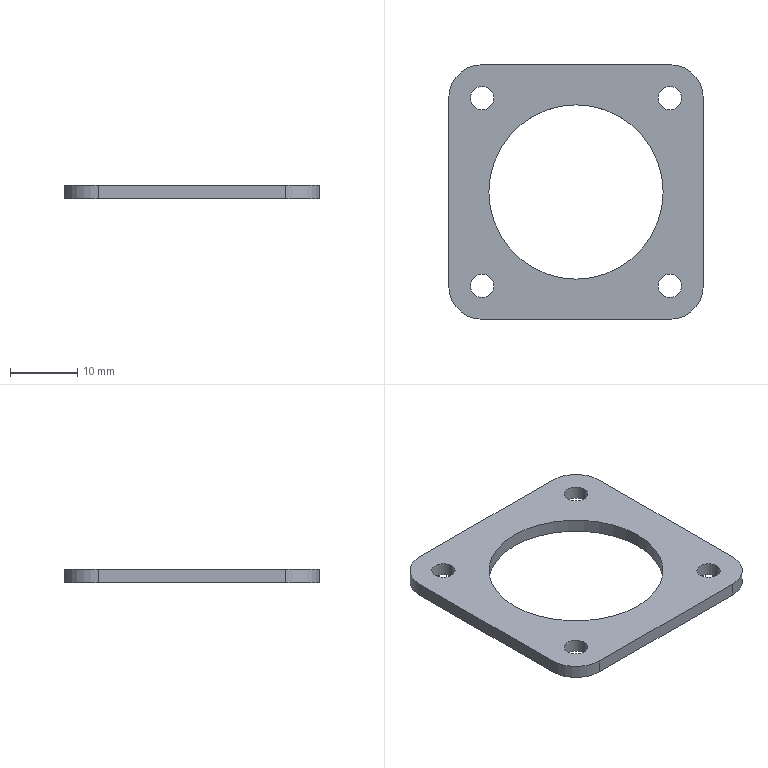Part | STEP file | bearing cover plate | 1 solid | 20 faces | box 38 x 38 x 2 mm | volume 1706 mm3 | cylinder 14 | plane 6 | commonest cylinder face diameters 3.5 x8 10 x4 26 x2